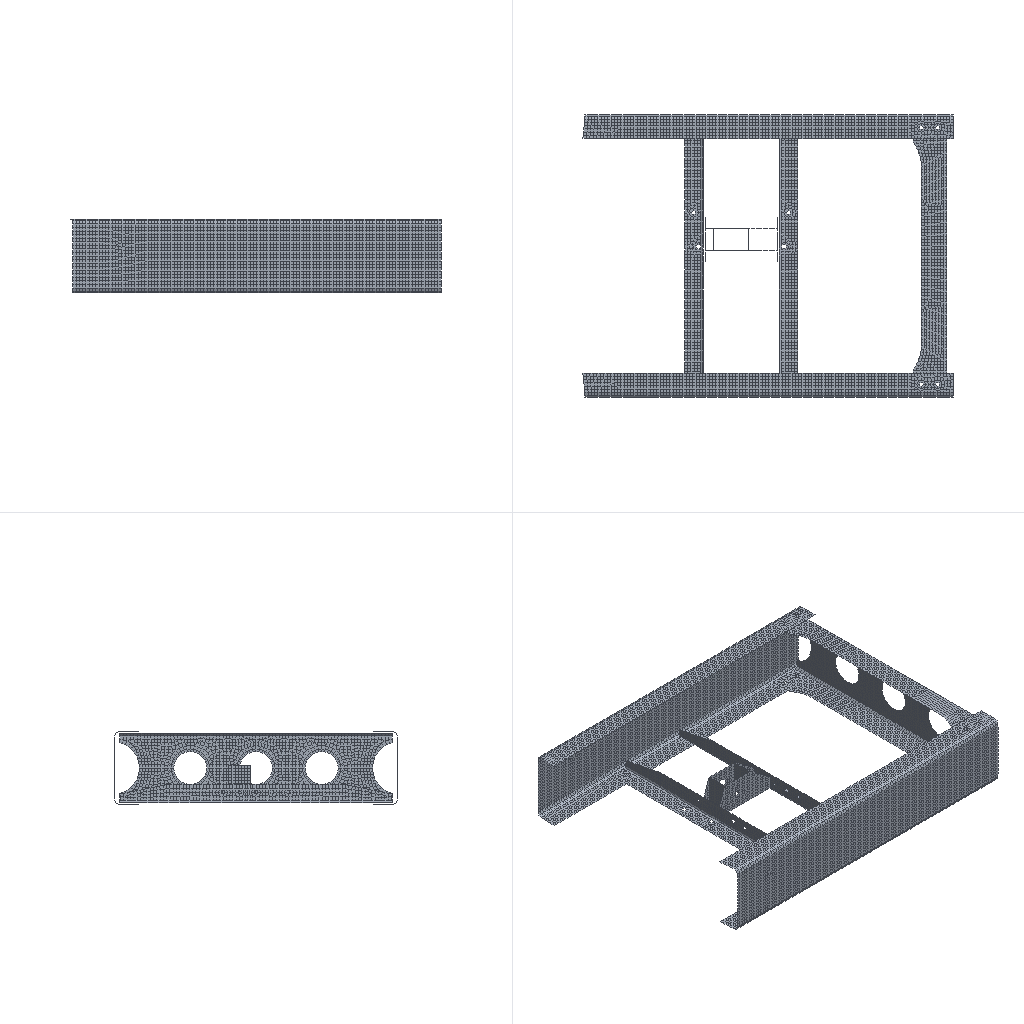Simulation study | nastran
Set-up summary:
category,name,step,type,value,unit,region
solver,nx_nastran
units,not stated in the deck,,not stated
analysis,deck,,static,static
analysis,solution,,SOL,101
load_step,SUBCASE 1,1,SUBCASE,SPC=6 LOAD=1
load_step,SUBCASE 2,2,SUBCASE,SPC=6 LOAD=2
load_step,SUBCASE 3,3,SUBCASE,SPC=6 LOAD=3
load_step,SUBCASE 4,4,SUBCASE,SPC=6 LOAD=4
load_step,requested,,,4
mesh,nodes,,,13959
mesh,elements,,,13162
element_type,CONM2,,mass,1
element_type,CQUAD4,,shell,13027
element_type,CTRIA3,,shell,134
load,load commands in deck,,count,4
bc,support commands in deck,,count,70
check,setup vs results,,match,"every grid point's frame and coordinates and every element id; grid points of CQUAD4, CTRIA3 elements"
Nastran input file, long lists of numbers shortened:
$$------------------------------------------------------------------------------$
$$                                                                              $
$$ NASTRAN Input Deck Generated by HyperMesh Version  : 9.0b121                 $
$$ Generated using HyperMesh-Nastran Template Version : 9.0b121
$$                                                                              $
$$   Template:  general                                                         $
$$                                                                              $
$$------------------------------------------------------------------------------$
$$------------------------------------------------------------------------------$
$$                      Executive Control Cards                                 $
$$------------------------------------------------------------------------------$
SOL 101
CEND
$$------------------------------------------------------------------------------$
$$                      Case Control Cards                                      $
$$------------------------------------------------------------------------------$
  DISPLACEMENT(PLOT) = ALL
  STRESS(PLOT) = ALL
  STRAIN(PLOT) = ALL
$
$HMNAME LOADSTEP               1"Step_X2g"
SUBCASE       1
  LABEL=    Step_X2g
  SPC =        6
  LOAD =        1
$
$HMNAME LOADSTEP               2"Step_Y2g"
SUBCASE       2
  LABEL=    Step_Y2g
  SPC =        6
  LOAD =        2
$
$HMNAME LOADSTEP               3"Step_Z2g"
SUBCASE       3
  LABEL=    Step_Z2g
  SPC =        6
  LOAD =        3
$
$HMNAME LOADSTEP               4"Step_Z-4g"
SUBCASE       4
  LABEL=    Step_Z-4g
  SPC =        6
  LOAD =        4
$$------------------------------------------------------------------------------$
$$                      Bulk Data Cards                                         $
$$------------------------------------------------------------------------------$
BEGIN BULK
PARAM,BAILOUT,-1
PARAM,POST,-1
$$
$$  GRID Data
$$
GRID         147        6993.33480.55083-221.5
GRID         148        7003.19771.13783-221.5
$ (13957 more lines like these left out)
$$
$$  SPOINT Data
$$
$
$  CONM2 Elements
$
CONM2     813744  846220       00.078   0.0     0.0     0.0
$
$HMMOVE 16070017
$         813744
$
$$
$$------------------------------------------------------------------------------$
$$             Group Definitions                                                $
$$------------------------------------------------------------------------------$
$$
$$ RBE2 Elements - Multiple dependent nodes
$$
RBE2      813725  846202  123456    2554  198348  198349  198350  198351+
+         198352  198796  198797  198798  198799  198800  198801  198802+
+         198803  198804  198805  198806  204941  204942  204943  204944+
+         204945  204946  204947  204948  204949  204950  204951  204952+
+         204953  204954  205000
RBE2      813726  846203  123456    2246    2257    2258    2259    2260+
+           2261    2262    2263    2264   95623   95624   95625   95626+
+          95627   96071   96072   96073   96074   96075   96076   96077+
+          96078   96079   96080   96081  204455  204456  204483  204499+
+         204500  204519  204845
$ (65 more lines like these left out)
$
$HMMOVE 16070016
$         813725THRU      813727  813729  813731THRU      813743
$
$$
$$  CTRIA3 Data
$$
CTRIA3     42242      12   42359   42357   42356
CTRIA3     42385      12   42477   42476   42473
$ (132 more lines like these left out)
$
$HMMOVE  2801012
$          42242   42385   42776   42805   42813   42821   42824   42837   42847
$          42856   42879THRU       42880   42891   42900THRU       42901   42929
$ (30 more lines like these left out)
CQUAD4     44848      12   44897   44867   44965   45215
CQUAD4     44849      12   45379   44866   45387   44876
$ (13025 more lines like these left out)
$
$HMMOVE  2801012
$          44848THRU       44853   44856THRU       44863   44865THRU       44874
$          44877THRU       44898   44900THRU       44907   44909THRU       44917
$ (277 more lines like these left out)
PSHELL         7      353.0           35              35
$
$HMNAME PROP                   9"Sheel_500T" 4
$HWCOLOR PROP                  9       5
PSHELL         9      355.0           35              35
$
$HMNAME PROP                  12"Sheel_600T" 4
$HWCOLOR PROP                 12       3
PSHELL        12      356.0           35              35
$$
$$------------------------------------------------------------------------------$
$$                      Material Definition Cards                               $
$$------------------------------------------------------------------------------$
$$--------------------------------------------------------------
$$ HYPERMESH TAGS
$$--------------------------------------------------------------
$$BEGIN TAGS
$$END TAGS
$$
$$  MAT1 Data
$
$HMNAME MAT                   35"steel" "MAT1"
$HWCOLOR MAT                  35       6
MAT1          35210000.0        0.3     7.80E-09
$$
$$
$$
$$------------------------------------------------------------------------------$
$ (27 more lines like these left out)
GRAV           1        9800.0  2.0     0.0     0.0
$$
$HMNAME LOADCOL                2"Y2g"
$HWCOLOR LOADCOL               2       4
GRAV           2        9800.0  0.0     2.0     0.0
$$
$HMNAME LOADCOL                3"Z2g"
$HWCOLOR LOADCOL               3       5
GRAV           3        9800.0  0.0     0.0     2.0
$$
$HMNAME LOADCOL                4"Z-4g"
$HWCOLOR LOADCOL               4       6
GRAV           4        9800.0  0.0     0.0     -4.0
$$
$$
$$
$$
$$
$$
$$
$$
$$
$$
$$
$$  SPC Data
$$
SPC            6  203088  1234560.0
SPC            6  203087  1234560.0
SPC            6  203086  1234560.0
SPC            6  203085  1234560.0
$ (66 more lines like these left out)
$
ENDDATA
Results summary:
result,analysis,,,static
result,last_loadstep,,,4
result,primary field,,,displacements
result,max displacement,,,0.8562,model units